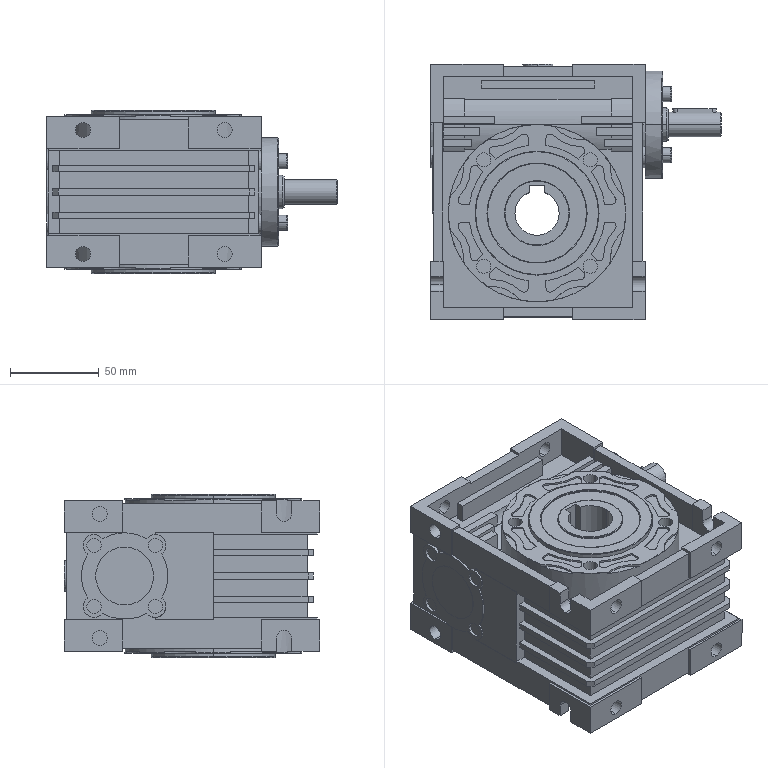Part | SolidWorks | features ICE 59, CirPattern 14, Fillet 9, Revolution 9, Chamfer 7, MirrorPattern 3, DeleteBody 2, RevCut 2, Extrusion 1, MirrorSolid 1, SketchPattern 1 | 1 solid | 694 faces | box 164 x 144 x 92 mm | volume 1188126 mm3 | plane 394 | cylinder 246 | torus 40 | cone 14 | commonest cylinder face diameters 4.802 x40 8.5 x34 38.734 x20 57.4 x18 8 x16 8.16 x16